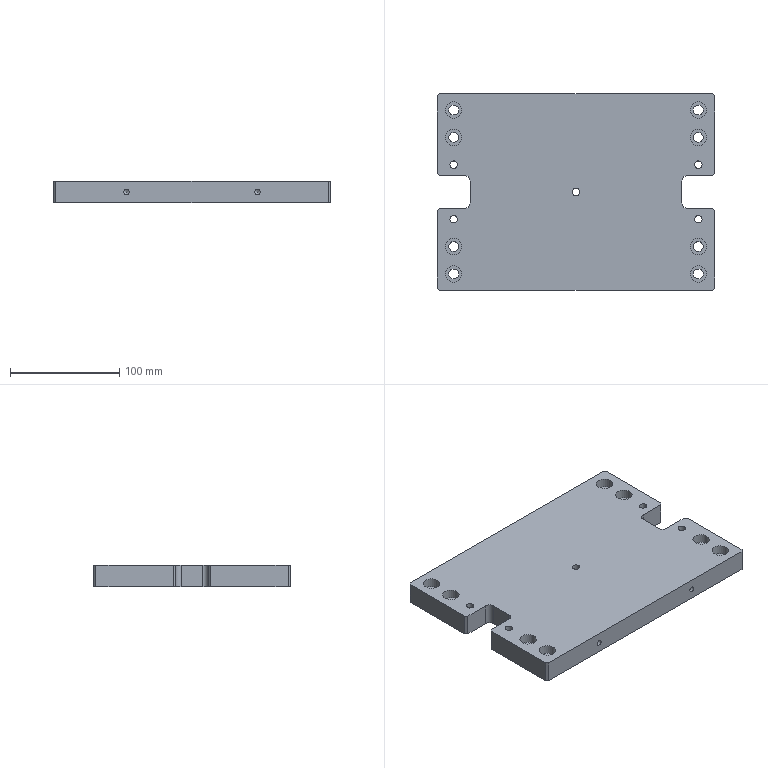Part | 1 solid | 63 faces | box 254 x 180 x 20 mm | volume 855700 mm3 | plane 30 | cylinder 29 | cone 4 | commonest cylinder face diameters 9 x8 15 x8 6.8 x5 5 x4 10 x4